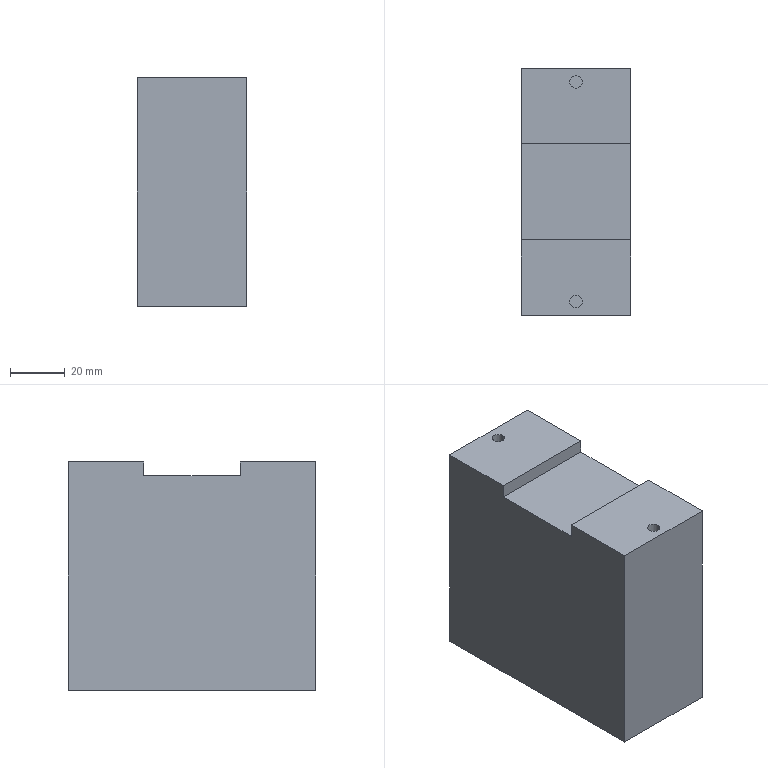Part | STEP file | BZJ-LSX-RGX PLC扩展IO FX5-16ET_ES8(输入,8输出,晶体管漏型) | 1 solid | 16 faces | box 40 x 90 x 83 mm | volume 291482 mm3 | plane 12 | cylinder 4 | commonest cylinder face diameters 4.5 x4
STEP:
#1=CARTESIAN_POINT('',(0.,0.,0.));
#2=DIRECTION('',(0.,0.,1.));
#3=DIRECTION('',(1.,0.,0.));
#4=AXIS2_PLACEMENT_3D('',#1,#2,#3);
#5=CARTESIAN_POINT('',(2.25,40.,31.5));
#6=VERTEX_POINT('',#5);
#7=CARTESIAN_POINT('',(2.25,40.,41.5));
#8=VERTEX_POINT('',#7);
#9=CARTESIAN_POINT('',(2.25,40.,31.5));
#10=DIRECTION('',(0.,0.,1.));
#11=VECTOR('',#10,1.);
#12=LINE('',#9,#11);
#13=CARTESIAN_POINT('',(0.,40.,31.5));
#14=DIRECTION('',(0.,0.,1.));
#15=DIRECTION('',(1.,0.,0.));
#16=AXIS2_PLACEMENT_3D('',#13,#14,#15);
#17=CYLINDRICAL_SURFACE('',#16,2.25);
#18=CARTESIAN_POINT('',(6.283,0.));
#19=DIRECTION('',(0.,1.));
#20=VECTOR('',#19,1.);
#21=LINE('',#18,#20);
#22=(GEOMETRIC_REPRESENTATION_CONTEXT(2)PARAMETRIC_REPRESENTATION_CONTEXT()REPRESENTATION_CONTEXT('',''));
#23=DEFINITIONAL_REPRESENTATION('',(#21),#22);
#24=PCURVE('',#17,#23);
#25=CARTESIAN_POINT('',(0.,40.,31.5));
#26=DIRECTION('',(0.,0.,1.));
#27=DIRECTION('',(1.,0.,0.));
#28=AXIS2_PLACEMENT_3D('',#25,#26,#27);
#29=CYLINDRICAL_SURFACE('',#28,2.25);
#30=CARTESIAN_POINT('',(0.,0.));
#31=DIRECTION('',(0.,1.));
#32=VECTOR('',#31,1.);
#33=LINE('',#30,#32);
#34=(GEOMETRIC_REPRESENTATION_CONTEXT(2)PARAMETRIC_REPRESENTATION_CONTEXT()REPRESENTATION_CONTEXT('',''));
#35=DEFINITIONAL_REPRESENTATION('',(#33),#34);
#36=PCURVE('',#29,#35);
#37=SURFACE_CURVE('',#12,(#24,#36),.PCURVE_S1.);
#38=EDGE_CURVE('',#6,#8,#37,.T.);
#39=ORIENTED_EDGE('',*,*,#38,.T.);
#40=CARTESIAN_POINT('',(-2.25,40.,41.5));
#41=VERTEX_POINT('',#40);
#42=CARTESIAN_POINT('',(0.,40.,41.5));
#43=DIRECTION('',(0.,0.,-1.));
#44=DIRECTION('',(-1.,0.,0.));
#45=AXIS2_PLACEMENT_3D('',#42,#43,#44);
#46=CIRCLE('',#45,2.25);
#47=CARTESIAN_POINT('',(9.425,10.));
#48=DIRECTION('',(-1.,0.));
#49=VECTOR('',#48,1.);
#50=LINE('',#47,#49);
#51=(GEOMETRIC_REPRESENTATION_CONTEXT(2)PARAMETRIC_REPRESENTATION_CONTEXT()REPRESENTATION_CONTEXT('',''));
#52=DEFINITIONAL_REPRESENTATION('',(#50),#51);
#53=PCURVE('',#17,#52);
#54=CARTESIAN_POINT('',(0.,0.,41.5));
#55=DIRECTION('',(0.,0.,-1.));
#56=DIRECTION('',(-1.,0.,0.));
#57=AXIS2_PLACEMENT_3D('',#54,#55,#56);
#58=PLANE('',#57);
#59=CARTESIAN_POINT('',(0.,40.));
#60=DIRECTION('',(1.,0.));
#61=AXIS2_PLACEMENT_2D('',#59,#60);
#62=CIRCLE('',#61,2.25);
#63=(GEOMETRIC_REPRESENTATION_CONTEXT(2)PARAMETRIC_REPRESENTATION_CONTEXT()REPRESENTATION_CONTEXT('',''));
#64=DEFINITIONAL_REPRESENTATION('',(#62),#63);
#65=PCURVE('',#58,#64);
#66=SURFACE_CURVE('',#46,(#53,#65),.PCURVE_S1.);
#67=EDGE_CURVE('',#8,#41,#66,.T.);
#68=ORIENTED_EDGE('',*,*,#67,.T.);
#69=CARTESIAN_POINT('',(-2.25,40.,31.5));
#70=VERTEX_POINT('',#69);
#71=CARTESIAN_POINT('',(-2.25,40.,31.5));
#72=DIRECTION('',(0.,0.,1.));
#73=VECTOR('',#72,1.);
#74=LINE('',#71,#73);
#75=CARTESIAN_POINT('',(3.142,0.));
#76=DIRECTION('',(0.,1.));
#77=VECTOR('',#76,1.);
#78=LINE('',#75,#77);
#79=(GEOMETRIC_REPRESENTATION_CONTEXT(2)PARAMETRIC_REPRESENTATION_CONTEXT()REPRESENTATION_CONTEXT('',''));
#80=DEFINITIONAL_REPRESENTATION('',(#78),#79);
#81=PCURVE('',#17,#80);
#82=CARTESIAN_POINT('',(3.142,0.));
#83=DIRECTION('',(0.,1.));
#84=VECTOR('',#83,1.);
#85=LINE('',#82,#84);
#86=(GEOMETRIC_REPRESENTATION_CONTEXT(2)PARAMETRIC_REPRESENTATION_CONTEXT()REPRESENTATION_CONTEXT('',''));
#87=DEFINITIONAL_REPRESENTATION('',(#85),#86);
#88=PCURVE('',#29,#87);
#89=SURFACE_CURVE('',#74,(#81,#88),.PCURVE_S1.);
#90=EDGE_CURVE('',#70,#41,#89,.T.);
#91=ORIENTED_EDGE('',*,*,#90,.F.);
#92=CARTESIAN_POINT('',(0.,40.,31.5));
#93=DIRECTION('',(0.,0.,-1.));
#94=DIRECTION('',(-1.,0.,0.));
#95=AXIS2_PLACEMENT_3D('',#92,#93,#94);
#96=CIRCLE('',#95,2.25);
#97=CARTESIAN_POINT('',(9.425,0.));
#98=DIRECTION('',(-1.,0.));
#99=VECTOR('',#98,1.);
#100=LINE('',#97,#99);
#101=(GEOMETRIC_REPRESENTATION_CONTEXT(2)PARAMETRIC_REPRESENTATION_CONTEXT()REPRESENTATION_CONTEXT('',''));
#102=DEFINITIONAL_REPRESENTATION('',(#100),#101);
#103=PCURVE('',#17,#102);
#104=CARTESIAN_POINT('',(0.,40.,31.5));
#105=DIRECTION('',(0.,0.,-1.));
#106=DIRECTION('',(-1.,0.,0.));
#107=AXIS2_PLACEMENT_3D('',#104,#105,#106);
#108=PLANE('',#107);
#109=CARTESIAN_POINT('',(0.,0.));
#110=DIRECTION('',(1.,0.));
#111=AXIS2_PLACEMENT_2D('',#109,#110);
#112=CIRCLE('',#111,2.25);
#113=(GEOMETRIC_REPRESENTATION_CONTEXT(2)PARAMETRIC_REPRESENTATION_CONTEXT()REPRESENTATION_CONTEXT('',''));
#114=DEFINITIONAL_REPRESENTATION('',(#112),#113);
#115=PCURVE('',#108,#114);
#116=SURFACE_CURVE('',#96,(#103,#115),.PCURVE_S1.);
#117=EDGE_CURVE('',#6,#70,#116,.T.);
#118=ORIENTED_EDGE('',*,*,#117,.F.);
#119=EDGE_LOOP('',(#39,#68,#91,#118));
#120=FACE_BOUND('',#119,.F.);
#121=ADVANCED_FACE('',(#120),#17,.F.);
#122=CARTESIAN_POINT('',(2.25,-40.,31.5));
#123=VERTEX_POINT('',#122);
#124=CARTESIAN_POINT('',(2.25,-40.,41.5));
#125=VERTEX_POINT('',#124);
#126=CARTESIAN_POINT('',(2.25,-40.,31.5));
#127=DIRECTION('',(0.,0.,1.));
#128=VECTOR('',#127,1.);
#129=LINE('',#126,#128);
#130=CARTESIAN_POINT('',(0.,-40.,31.5));
#131=DIRECTION('',(0.,0.,1.));
#132=DIRECTION('',(1.,0.,0.));
#133=AXIS2_PLACEMENT_3D('',#130,#131,#132);
#134=CYLINDRICAL_SURFACE('',#133,2.25);
#135=CARTESIAN_POINT('',(6.283,0.));
#136=DIRECTION('',(0.,1.));
#137=VECTOR('',#136,1.);
#138=LINE('',#135,#137);
#139=(GEOMETRIC_REPRESENTATION_CONTEXT(2)PARAMETRIC_REPRESENTATION_CONTEXT()REPRESENTATION_CONTEXT('',''));
#140=DEFINITIONAL_REPRESENTATION('',(#138),#139);
#141=PCURVE('',#134,#140);
#142=CARTESIAN_POINT('',(0.,-40.,31.5));
#143=DIRECTION('',(0.,0.,1.));
#144=DIRECTION('',(1.,0.,0.));
#145=AXIS2_PLACEMENT_3D('',#142,#143,#144);
#146=CYLINDRICAL_SURFACE('',#145,2.25);
#147=CARTESIAN_POINT('',(0.,0.));
#148=DIRECTION('',(0.,1.));
#149=VECTOR('',#148,1.);
#150=LINE('',#147,#149);
#151=(GEOMETRIC_REPRESENTATION_CONTEXT(2)PARAMETRIC_REPRESENTATION_CONTEXT()REPRESENTATION_CONTEXT('',''));
#152=DEFINITIONAL_REPRESENTATION('',(#150),#151);
#153=PCURVE('',#146,#152);
#154=SURFACE_CURVE('',#129,(#141,#153),.PCURVE_S1.);
#155=EDGE_CURVE('',#123,#125,#154,.T.);
#156=ORIENTED_EDGE('',*,*,#155,.T.);
#157=CARTESIAN_POINT('',(-2.25,-40.,41.5));
#158=VERTEX_POINT('',#157);
#159=CARTESIAN_POINT('',(0.,-40.,41.5));
#160=DIRECTION('',(0.,0.,-1.));
#161=DIRECTION('',(1.,0.,0.));
#162=AXIS2_PLACEMENT_3D('',#159,#160,#161);
#163=CIRCLE('',#162,2.25);
#164=CARTESIAN_POINT('',(6.283,10.));
#165=DIRECTION('',(-1.,0.));
#166=VECTOR('',#165,1.);
#167=LINE('',#164,#166);
#168=(GEOMETRIC_REPRESENTATION_CONTEXT(2)PARAMETRIC_REPRESENTATION_CONTEXT()REPRESENTATION_CONTEXT('',''));
#169=DEFINITIONAL_REPRESENTATION('',(#167),#168);
#170=PCURVE('',#134,#169);
#171=CARTESIAN_POINT('',(0.,0.,41.5));
#172=DIRECTION('',(0.,0.,-1.));
#173=DIRECTION('',(-1.,0.,0.));
#174=AXIS2_PLACEMENT_3D('',#171,#172,#173);
#175=PLANE('',#174);
#176=CARTESIAN_POINT('',(0.,-40.));
#177=DIRECTION('',(-1.,0.));
#178=AXIS2_PLACEMENT_2D('',#176,#177);
#179=CIRCLE('',#178,2.25);
#180=(GEOMETRIC_REPRESENTATION_CONTEXT(2)PARAMETRIC_REPRESENTATION_CONTEXT()REPRESENTATION_CONTEXT('',''));
#181=DEFINITIONAL_REPRESENTATION('',(#179),#180);
#182=PCURVE('',#175,#181);
#183=SURFACE_CURVE('',#163,(#170,#182),.PCURVE_S1.);
#184=EDGE_CURVE('',#125,#158,#183,.T.);
#185=ORIENTED_EDGE('',*,*,#184,.T.);
#186=CARTESIAN_POINT('',(-2.25,-40.,31.5));
#187=VERTEX_POINT('',#186);
#188=CARTESIAN_POINT('',(-2.25,-40.,31.5));
#189=DIRECTION('',(0.,0.,1.));
#190=VECTOR('',#189,1.);
#191=LINE('',#188,#190);
#192=CARTESIAN_POINT('',(3.142,0.));
#193=DIRECTION('',(0.,1.));
#194=VECTOR('',#193,1.);
#195=LINE('',#192,#194);
#196=(GEOMETRIC_REPRESENTATION_CONTEXT(2)PARAMETRIC_REPRESENTATION_CONTEXT()REPRESENTATION_CONTEXT('',''));
#197=DEFINITIONAL_REPRESENTATION('',(#195),#196);
#198=PCURVE('',#134,#197);
#199=CARTESIAN_POINT('',(3.142,0.));
#200=DIRECTION('',(0.,1.));
#201=VECTOR('',#200,1.);
#202=LINE('',#199,#201);
#203=(GEOMETRIC_REPRESENTATION_CONTEXT(2)PARAMETRIC_REPRESENTATION_CONTEXT()REPRESENTATION_CONTEXT('',''));
#204=DEFINITIONAL_REPRESENTATION('',(#202),#203);
#205=PCURVE('',#146,#204);
#206=SURFACE_CURVE('',#191,(#198,#205),.PCURVE_S1.);
#207=EDGE_CURVE('',#187,#158,#206,.T.);
#208=ORIENTED_EDGE('',*,*,#207,.F.);
#209=CARTESIAN_POINT('',(0.,-40.,31.5));
#210=DIRECTION('',(0.,0.,-1.));
#211=DIRECTION('',(1.,0.,0.));
#212=AXIS2_PLACEMENT_3D('',#209,#210,#211);
#213=CIRCLE('',#212,2.25);
#214=CARTESIAN_POINT('',(6.283,0.));
#215=DIRECTION('',(-1.,0.));
#216=VECTOR('',#215,1.);
#217=LINE('',#214,#216);
#218=(GEOMETRIC_REPRESENTATION_CONTEXT(2)PARAMETRIC_REPRESENTATION_CONTEXT()REPRESENTATION_CONTEXT('',''));
#219=DEFINITIONAL_REPRESENTATION('',(#217),#218);
#220=PCURVE('',#134,#219);
#221=CARTESIAN_POINT('',(0.,-40.,31.5));
#222=DIRECTION('',(0.,0.,1.));
#223=DIRECTION('',(1.,0.,0.));
#224=AXIS2_PLACEMENT_3D('',#221,#222,#223);
#225=PLANE('',#224);
#226=CARTESIAN_POINT('',(2.25,0.));
#227=CARTESIAN_POINT('',(2.25,-3.897));
#228=CARTESIAN_POINT('',(-1.125,-1.949));
#229=CARTESIAN_POINT('',(-4.5,0.));
#230=CARTESIAN_POINT('',(-1.125,1.949));
#231=CARTESIAN_POINT('',(2.25,3.897));
#232=CARTESIAN_POINT('',(2.25,0.));
#233=(BOUNDED_CURVE()B_SPLINE_CURVE(2,(#226,#227,#228,#229,#230,#231,#232),.UNSPECIFIED.,.T.,.F.)B_SPLINE_CURVE_WITH_KNOTS((1,2,2,2,2,1),(-2.094,0.,2.094,4.189,6.283,8.378),.UNSPECIFIED.)CURVE()GEOMETRIC_REPRESENTATION_ITEM()RATIONAL_B_SPLINE_CURVE((1.,0.5,1.,0.5,1.,0.5,1.))REPRESENTATION_ITEM(''));
#234=(GEOMETRIC_REPRESENTATION_CONTEXT(2)PARAMETRIC_REPRESENTATION_CONTEXT()REPRESENTATION_CONTEXT('',''));
#235=DEFINITIONAL_REPRESENTATION('',(#233),#234);
#236=PCURVE('',#225,#235);
#237=SURFACE_CURVE('',#213,(#220,#236),.PCURVE_S1.);
#238=EDGE_CURVE('',#123,#187,#237,.T.);
#239=ORIENTED_EDGE('',*,*,#238,.F.);
#240=EDGE_LOOP('',(#156,#185,#208,#239));
#241=FACE_BOUND('',#240,.F.);
#242=ADVANCED_FACE('',(#241),#134,.F.);
#243=ORIENTED_EDGE('',*,*,#67,.T.);
#244=CARTESIAN_POINT('',(0.,40.,41.5));
#245=DIRECTION('',(0.,0.,-1.));
#246=DIRECTION('',(-1.,0.,0.));
#247=AXIS2_PLACEMENT_3D('',#244,#245,#246);
#248=CIRCLE('',#247,2.25);
#249=CARTESIAN_POINT('',(0.,40.));
#250=DIRECTION('',(1.,0.));
#251=AXIS2_PLACEMENT_2D('',#249,#250);
#252=CIRCLE('',#251,2.25);
#253=(GEOMETRIC_REPRESENTATION_CONTEXT(2)PARAMETRIC_REPRESENTATION_CONTEXT()REPRESENTATION_CONTEXT('',''));
#254=DEFINITIONAL_REPRESENTATION('',(#252),#253);
#255=PCURVE('',#58,#254);
#256=CARTESIAN_POINT('',(3.142,10.));
#257=DIRECTION('',(-1.,0.));
#258=VECTOR('',#257,1.);
#259=LINE('',#256,#258);
#260=(GEOMETRIC_REPRESENTATION_CONTEXT(2)PARAMETRIC_REPRESENTATION_CONTEXT()REPRESENTATION_CONTEXT('',''));
#261=DEFINITIONAL_REPRESENTATION('',(#259),#260);
#262=PCURVE('',#29,#261);
#263=SURFACE_CURVE('',#248,(#255,#262),.PCURVE_S1.);
#264=EDGE_CURVE('',#41,#8,#263,.T.);
#265=ORIENTED_EDGE('',*,*,#264,.T.);
#266=EDGE_LOOP('',(#243,#265));
#267=FACE_BOUND('',#266,.T.);
#268=CARTESIAN_POINT('',(-20.,45.,41.5));
#269=VERTEX_POINT('',#268);
#270=CARTESIAN_POINT('',(-20.,17.5,41.5));
#271=VERTEX_POINT('',#270);
#272=CARTESIAN_POINT('',(-20.,45.,41.5));
#273=DIRECTION('',(0.,-1.,0.));
#274=VECTOR('',#273,1.);
#275=LINE('',#272,#274);
#276=CARTESIAN_POINT('',(20.,45.));
#277=DIRECTION('',(0.,-1.));
#278=VECTOR('',#277,1.);
#279=LINE('',#276,#278);
#280=(GEOMETRIC_REPRESENTATION_CONTEXT(2)PARAMETRIC_REPRESENTATION_CONTEXT()REPRESENTATION_CONTEXT('',''));
#281=DEFINITIONAL_REPRESENTATION('',(#279),#280);
#282=PCURVE('',#58,#281);
#283=CARTESIAN_POINT('',(-20.,45.,41.5));
#284=DIRECTION('',(1.,0.,0.));
#285=DIRECTION('',(0.,1.,0.));
#286=AXIS2_PLACEMENT_3D('',#283,#284,#285);
#287=PLANE('',#286);
#288=CARTESIAN_POINT('',(0.,0.));
#289=DIRECTION('',(-1.,0.));
#290=VECTOR('',#289,1.);
#291=LINE('',#288,#290);
#292=(GEOMETRIC_REPRESENTATION_CONTEXT(2)PARAMETRIC_REPRESENTATION_CONTEXT()REPRESENTATION_CONTEXT('',''));
#293=DEFINITIONAL_REPRESENTATION('',(#291),#292);
#294=PCURVE('',#287,#293);
#295=SURFACE_CURVE('',#275,(#282,#294),.PCURVE_S1.);
#296=EDGE_CURVE('',#269,#271,#295,.T.);
#297=ORIENTED_EDGE('',*,*,#296,.T.);
#298=CARTESIAN_POINT('',(20.,17.5,41.5));
#299=VERTEX_POINT('',#298);
#300=CARTESIAN_POINT('',(0.,17.5,41.5));
#301=DIRECTION('',(1.,0.,0.));
#302=VECTOR('',#301,1.);
#303=LINE('',#300,#302);
#304=CARTESIAN_POINT('',(0.,17.5));
#305=DIRECTION('',(-1.,0.));
#306=VECTOR('',#305,1.);
#307=LINE('',#304,#306);
#308=(GEOMETRIC_REPRESENTATION_CONTEXT(2)PARAMETRIC_REPRESENTATION_CONTEXT()REPRESENTATION_CONTEXT('',''));
#309=DEFINITIONAL_REPRESENTATION('',(#307),#308);
#310=PCURVE('',#58,#309);
#311=CARTESIAN_POINT('',(-20.,17.5,36.5));
#312=DIRECTION('',(0.,1.,0.));
#313=DIRECTION('',(-1.,0.,0.));
#314=AXIS2_PLACEMENT_3D('',#311,#312,#313);
#315=PLANE('',#314);
#316=CARTESIAN_POINT('',(-20.,5.));
#317=DIRECTION('',(-1.,0.));
#318=VECTOR('',#317,1.);
#319=LINE('',#316,#318);
#320=(GEOMETRIC_REPRESENTATION_CONTEXT(2)PARAMETRIC_REPRESENTATION_CONTEXT()REPRESENTATION_CONTEXT('',''));
#321=DEFINITIONAL_REPRESENTATION('',(#319),#320);
#322=PCURVE('',#315,#321);
#323=SURFACE_CURVE('',#303,(#310,#322),.PCURVE_S1.);
#324=EDGE_CURVE('',#271,#299,#323,.T.);
#325=ORIENTED_EDGE('',*,*,#324,.T.);
#326=CARTESIAN_POINT('',(20.,45.,41.5));
#327=VERTEX_POINT('',#326);
#328=CARTESIAN_POINT('',(20.,45.,41.5));
#329=DIRECTION('',(0.,1.,0.));
#330=VECTOR('',#329,1.);
#331=LINE('',#328,#330);
#332=CARTESIAN_POINT('',(-20.,45.));
#333=DIRECTION('',(0.,1.));
#334=VECTOR('',#333,1.);
#335=LINE('',#332,#334);
#336=(GEOMETRIC_REPRESENTATION_CONTEXT(2)PARAMETRIC_REPRESENTATION_CONTEXT()REPRESENTATION_CONTEXT('',''));
#337=DEFINITIONAL_REPRESENTATION('',(#335),#336);
#338=PCURVE('',#58,#337);
#339=CARTESIAN_POINT('',(20.,45.,41.5));
#340=DIRECTION('',(-1.,0.,0.));
#341=DIRECTION('',(0.,-1.,0.));
#342=AXIS2_PLACEMENT_3D('',#339,#340,#341);
#343=PLANE('',#342);
#344=CARTESIAN_POINT('',(0.,0.));
#345=DIRECTION('',(-1.,0.));
#346=VECTOR('',#345,1.);
#347=LINE('',#344,#346);
#348=(GEOMETRIC_REPRESENTATION_CONTEXT(2)PARAMETRIC_REPRESENTATION_CONTEXT()REPRESENTATION_CONTEXT('',''));
#349=DEFINITIONAL_REPRESENTATION('',(#347),#348);
#350=PCURVE('',#343,#349);
#351=SURFACE_CURVE('',#331,(#338,#350),.PCURVE_S1.);
#352=EDGE_CURVE('',#299,#327,#351,.T.);
#353=ORIENTED_EDGE('',*,*,#352,.T.);
#354=CARTESIAN_POINT('',(20.,45.,41.5));
#355=DIRECTION('',(-1.,0.,0.));
#356=VECTOR('',#355,1.);
#357=LINE('',#354,#356);
#358=CARTESIAN_POINT('',(-20.,45.));
#359=DIRECTION('',(1.,0.));
#360=VECTOR('',#359,1.);
#361=LINE('',#358,#360);
#362=(GEOMETRIC_REPRESENTATION_CONTEXT(2)PARAMETRIC_REPRESENTATION_CONTEXT()REPRESENTATION_CONTEXT('',''));
#363=DEFINITIONAL_REPRESENTATION('',(#361),#362);
#364=PCURVE('',#58,#363);
#365=CARTESIAN_POINT('',(20.,45.,41.5));
#366=DIRECTION('',(0.,-1.,0.));
#367=DIRECTION('',(0.,0.,-1.));
#368=AXIS2_PLACEMENT_3D('',#365,#366,#367);
#369=PLANE('',#368);
#370=CARTESIAN_POINT('',(0.,0.));
#371=DIRECTION('',(0.,-1.));
#372=VECTOR('',#371,1.);
#373=LINE('',#370,#372);
#374=(GEOMETRIC_REPRESENTATION_CONTEXT(2)PARAMETRIC_REPRESENTATION_CONTEXT()REPRESENTATION_CONTEXT('',''));
#375=DEFINITIONAL_REPRESENTATION('',(#373),#374);
#376=PCURVE('',#369,#375);
#377=SURFACE_CURVE('',#357,(#364,#376),.PCURVE_S1.);
#378=EDGE_CURVE('',#327,#269,#377,.T.);
#379=ORIENTED_EDGE('',*,*,#378,.T.);
#380=EDGE_LOOP('',(#297,#325,#353,#379));
#381=FACE_BOUND('',#380,.T.);
#382=ADVANCED_FACE('',(#267,#381),#58,.F.);
#383=CARTESIAN_POINT('',(-20.,-17.5,36.5));
#384=VERTEX_POINT('',#383);
#385=CARTESIAN_POINT('',(-20.,17.5,36.5));
#386=VERTEX_POINT('',#385);
#387=CARTESIAN_POINT('',(-20.,17.5,36.5));
#388=DIRECTION('',(0.,1.,0.));
#389=VECTOR('',#388,1.);
#390=LINE('',#387,#389);
#391=CARTESIAN_POINT('',(-27.5,-5.));
#392=DIRECTION('',(1.,0.));
#393=VECTOR('',#392,1.);
#394=LINE('',#391,#393);
#395=(GEOMETRIC_REPRESENTATION_CONTEXT(2)PARAMETRIC_REPRESENTATION_CONTEXT()REPRESENTATION_CONTEXT('',''));
#396=DEFINITIONAL_REPRESENTATION('',(#394),#395);
#397=PCURVE('',#287,#396);
#398=CARTESIAN_POINT('',(-20.,17.5,36.5));
#399=DIRECTION('',(0.,0.,-1.));
#400=DIRECTION('',(-1.,0.,0.));
#401=AXIS2_PLACEMENT_3D('',#398,#399,#400);
#402=PLANE('',#401);
#403=CARTESIAN_POINT('',(0.,0.));
#404=DIRECTION('',(0.,1.));
#405=VECTOR('',#404,1.);
#406=LINE('',#403,#405);
#407=(GEOMETRIC_REPRESENTATION_CONTEXT(2)PARAMETRIC_REPRESENTATION_CONTEXT()REPRESENTATION_CONTEXT('',''));
#408=DEFINITIONAL_REPRESENTATION('',(#406),#407);
#409=PCURVE('',#402,#408);
#410=SURFACE_CURVE('',#390,(#397,#409),.PCURVE_S1.);
#411=EDGE_CURVE('',#384,#386,#410,.T.);
#412=ORIENTED_EDGE('',*,*,#411,.T.);
#413=CARTESIAN_POINT('',(-20.,17.5,36.5));
#414=DIRECTION('',(0.,0.,1.));
#415=VECTOR('',#414,1.);
#416=LINE('',#413,#415);
#417=CARTESIAN_POINT('',(-27.5,-5.));
#418=DIRECTION('',(0.,1.));
#419=VECTOR('',#418,1.);
#420=LINE('',#417,#419);
#421=(GEOMETRIC_REPRESENTATION_CONTEXT(2)PARAMETRIC_REPRESENTATION_CONTEXT()REPRESENTATION_CONTEXT('',''));
#422=DEFINITIONAL_REPRESENTATION('',(#420),#421);
#423=PCURVE('',#287,#422);
#424=CARTESIAN_POINT('',(0.,0.));
#425=DIRECTION('',(0.,1.));
#426=VECTOR('',#425,1.);
#427=LINE('',#424,#426);
#428=(GEOMETRIC_REPRESENTATION_CONTEXT(2)PARAMETRIC_REPRESENTATION_CONTEXT()REPRESENTATION_CONTEXT('',''));
#429=DEFINITIONAL_REPRESENTATION('',(#427),#428);
#430=PCURVE('',#315,#429);
#431=SURFACE_CURVE('',#416,(#423,#430),.PCURVE_S1.);
#432=EDGE_CURVE('',#386,#271,#431,.T.);
#433=ORIENTED_EDGE('',*,*,#432,.T.);
#434=ORIENTED_EDGE('',*,*,#296,.F.);
#435=CARTESIAN_POINT('',(-20.,45.,-41.5));
#436=VERTEX_POINT('',#435);
#437=CARTESIAN_POINT('',(-20.,45.,41.5));
#438=DIRECTION('',(0.,0.,-1.));
#439=VECTOR('',#438,1.);
#440=LINE('',#437,#439);
#441=CARTESIAN_POINT('',(0.,0.));
#442=DIRECTION('',(0.,-1.));
#443=VECTOR('',#442,1.);
#444=LINE('',#441,#443);
#445=(GEOMETRIC_REPRESENTATION_CONTEXT(2)PARAMETRIC_REPRESENTATION_CONTEXT()REPRESENTATION_CONTEXT('',''));
#446=DEFINITIONAL_REPRESENTATION('',(#444),#445);
#447=PCURVE('',#287,#446);
#448=CARTESIAN_POINT('',(0.,-40.));
#449=DIRECTION('',(1.,0.));
#450=VECTOR('',#449,1.);
#451=LINE('',#448,#450);
#452=(GEOMETRIC_REPRESENTATION_CONTEXT(2)PARAMETRIC_REPRESENTATION_CONTEXT()REPRESENTATION_CONTEXT('',''));
#453=DEFINITIONAL_REPRESENTATION('',(#451),#452);
#454=PCURVE('',#369,#453);
#455=SURFACE_CURVE('',#440,(#447,#454),.PCURVE_S1.);
#456=EDGE_CURVE('',#269,#436,#455,.T.);
#457=ORIENTED_EDGE('',*,*,#456,.T.);
#458=CARTESIAN_POINT('',(-20.,-45.,-41.5));
#459=VERTEX_POINT('',#458);
#460=CARTESIAN_POINT('',(-20.,45.,-41.5));
#461=DIRECTION('',(0.,-1.,0.));
#462=VECTOR('',#461,1.);
#463=LINE('',#460,#462);
#464=CARTESIAN_POINT('',(0.,-83.));
#465=DIRECTION('',(-1.,0.));
#466=VECTOR('',#465,1.);
#467=LINE('',#464,#466);
#468=(GEOMETRIC_REPRESENTATION_CONTEXT(2)PARAMETRIC_REPRESENTATION_CONTEXT()REPRESENTATION_CONTEXT('',''));
#469=DEFINITIONAL_REPRESENTATION('',(#467),#468);
#470=PCURVE('',#287,#469);
#471=CARTESIAN_POINT('',(0.,0.,-41.5));
#472=DIRECTION('',(0.,0.,-1.));
#473=DIRECTION('',(-1.,0.,0.));
#474=AXIS2_PLACEMENT_3D('',#471,#472,#473);
#475=PLANE('',#474);
#476=CARTESIAN_POINT('',(20.,45.));
#477=DIRECTION('',(0.,-1.));
#478=VECTOR('',#477,1.);
#479=LINE('',#476,#478);
#480=(GEOMETRIC_REPRESENTATION_CONTEXT(2)PARAMETRIC_REPRESENTATION_CONTEXT()REPRESENTATION_CONTEXT('',''));
#481=DEFINITIONAL_REPRESENTATION('',(#479),#480);
#482=PCURVE('',#475,#481);
#483=SURFACE_CURVE('',#463,(#470,#482),.PCURVE_S1.);
#484=EDGE_CURVE('',#436,#459,#483,.T.);
#485=ORIENTED_EDGE('',*,*,#484,.T.);
#486=CARTESIAN_POINT('',(-20.,-45.,41.5));
#487=VERTEX_POINT('',#486);
#488=CARTESIAN_POINT('',(-20.,-45.,41.5));
#489=DIRECTION('',(0.,0.,-1.));
#490=VECTOR('',#489,1.);
#491=LINE('',#488,#490);
#492=CARTESIAN_POINT('',(-90.,0.));
#493=DIRECTION('',(0.,-1.));
#494=VECTOR('',#493,1.);
#495=LINE('',#492,#494);
#496=(GEOMETRIC_REPRESENTATION_CONTEXT(2)PARAMETRIC_REPRESENTATION_CONTEXT()REPRESENTATION_CONTEXT('',''));
#497=DEFINITIONAL_REPRESENTATION('',(#495),#496);
#498=PCURVE('',#287,#497);
#499=CARTESIAN_POINT('',(20.,-45.,41.5));
#500=DIRECTION('',(0.,1.,0.));
#501=DIRECTION('',(-1.,0.,0.));
#502=AXIS2_PLACEMENT_3D('',#499,#500,#501);
#503=PLANE('',#502);
#504=CARTESIAN_POINT('',(40.,0.));
#505=DIRECTION('',(0.,-1.));
#506=VECTOR('',#505,1.);
#507=LINE('',#504,#506);
#508=(GEOMETRIC_REPRESENTATION_CONTEXT(2)PARAMETRIC_REPRESENTATION_CONTEXT()REPRESENTATION_CONTEXT('',''));
#509=DEFINITIONAL_REPRESENTATION('',(#507),#508);
#510=PCURVE('',#503,#509);
#511=SURFACE_CURVE('',#491,(#498,#510),.PCURVE_S1.);
#512=EDGE_CURVE('',#487,#459,#511,.T.);
#513=ORIENTED_EDGE('',*,*,#512,.F.);
#514=CARTESIAN_POINT('',(-20.,-17.5,41.5));
#515=VERTEX_POINT('',#514);
#516=CARTESIAN_POINT('',(-20.,45.,41.5));
#517=DIRECTION('',(0.,-1.,0.));
#518=VECTOR('',#517,1.);
#519=LINE('',#516,#518);
#520=CARTESIAN_POINT('',(0.,0.));
#521=DIRECTION('',(-1.,0.));
#522=VECTOR('',#521,1.);
#523=LINE('',#520,#522);
#524=(GEOMETRIC_REPRESENTATION_CONTEXT(2)PARAMETRIC_REPRESENTATION_CONTEXT()REPRESENTATION_CONTEXT('',''));
#525=DEFINITIONAL_REPRESENTATION('',(#523),#524);
#526=PCURVE('',#287,#525);
#527=CARTESIAN_POINT('',(20.,45.));
#528=DIRECTION('',(0.,-1.));
#529=VECTOR('',#528,1.);
#530=LINE('',#527,#529);
#531=(GEOMETRIC_REPRESENTATION_CONTEXT(2)PARAMETRIC_REPRESENTATION_CONTEXT()REPRESENTATION_CONTEXT('',''));
#532=DEFINITIONAL_REPRESENTATION('',(#530),#531);
#533=PCURVE('',#175,#532);
#534=SURFACE_CURVE('',#519,(#526,#533),.PCURVE_S1.);
#535=EDGE_CURVE('',#515,#487,#534,.T.);
#536=ORIENTED_EDGE('',*,*,#535,.F.);
#537=CARTESIAN_POINT('',(-20.,-17.5,36.5));
#538=DIRECTION('',(0.,0.,-1.));
#539=VECTOR('',#538,1.);
#540=LINE('',#537,#539);
#541=CARTESIAN_POINT('',(-62.5,-5.));
#542=DIRECTION('',(0.,-1.));
#543=VECTOR('',#542,1.);
#544=LINE('',#541,#543);
#545=(GEOMETRIC_REPRESENTATION_CONTEXT(2)PARAMETRIC_REPRESENTATION_CONTEXT()REPRESENTATION_CONTEXT('',''));
#546=DEFINITIONAL_REPRESENTATION('',(#544),#545);
#547=PCURVE('',#287,#546);
#548=CARTESIAN_POINT('',(-20.,-17.5,36.5));
#549=DIRECTION('',(0.,-1.,0.));
#550=DIRECTION('',(1.,0.,0.));
#551=AXIS2_PLACEMENT_3D('',#548,#549,#550);
#552=PLANE('',#551);
#553=CARTESIAN_POINT('',(0.,0.));
#554=DIRECTION('',(0.,-1.));
#555=VECTOR('',#554,1.);
#556=LINE('',#553,#555);
#557=(GEOMETRIC_REPRESENTATION_CONTEXT(2)PARAMETRIC_REPRESENTATION_CONTEXT()REPRESENTATION_CONTEXT('',''));
#558=DEFINITIONAL_REPRESENTATION('',(#556),#557);
#559=PCURVE('',#552,#558);
#560=SURFACE_CURVE('',#540,(#547,#559),.PCURVE_S1.);
#561=EDGE_CURVE('',#515,#384,#560,.T.);
#562=ORIENTED_EDGE('',*,*,#561,.T.);
#563=EDGE_LOOP('',(#412,#433,#434,#457,#485,#513,#536,#562));
#564=FACE_BOUND('',#563,.T.);
#565=ADVANCED_FACE('',(#564),#287,.F.);
#566=CARTESIAN_POINT('',(20.,-45.,-41.5));
#567=VERTEX_POINT('',#566);
#568=CARTESIAN_POINT('',(20.,-45.,-41.5));
#569=DIRECTION('',(1.,0.,0.));
#570=VECTOR('',#569,1.);
#571=LINE('',#568,#570);
#572=CARTESIAN_POINT('',(0.,-83.));
#573=DIRECTION('',(-1.,0.));
#574=VECTOR('',#573,1.);
#575=LINE('',#572,#574);
#576=(GEOMETRIC_REPRESENTATION_CONTEXT(2)PARAMETRIC_REPRESENTATION_CONTEXT()REPRESENTATION_CONTEXT('',''));
#577=DEFINITIONAL_REPRESENTATION('',(#575),#576);
#578=PCURVE('',#503,#577);
#579=CARTESIAN_POINT('',(-20.,-45.));
#580=DIRECTION('',(-1.,0.));
#581=VECTOR('',#580,1.);
#582=LINE('',#579,#581);
#583=(GEOMETRIC_REPRESENTATION_CONTEXT(2)PARAMETRIC_REPRESENTATION_CONTEXT()REPRESENTATION_CONTEXT('',''));
#584=DEFINITIONAL_REPRESENTATION('',(#582),#583);
#585=PCURVE('',#475,#584);
#586=SURFACE_CURVE('',#571,(#578,#585),.PCURVE_S1.);
#587=EDGE_CURVE('',#459,#567,#586,.T.);
#588=ORIENTED_EDGE('',*,*,#587,.T.);
#589=CARTESIAN_POINT('',(20.,-45.,41.5));
#590=VERTEX_POINT('',#589);
#591=CARTESIAN_POINT('',(20.,-45.,41.5));
#592=DIRECTION('',(0.,0.,-1.));
#593=VECTOR('',#592,1.);
#594=LINE('',#591,#593);
#595=CARTESIAN_POINT('',(0.,0.));
#596=DIRECTION('',(0.,-1.));
#597=VECTOR('',#596,1.);
#598=LINE('',#595,#597);
#599=(GEOMETRIC_REPRESENTATION_CONTEXT(2)PARAMETRIC_REPRESENTATION_CONTEXT()REPRESENTATION_CONTEXT('',''));
#600=DEFINITIONAL_REPRESENTATION('',(#598),#599);
#601=PCURVE('',#503,#600);
#602=CARTESIAN_POINT('',(90.,0.));
#603=DIRECTION('',(0.,-1.));
#604=VECTOR('',#603,1.);
#605=LINE('',#602,#604);
#606=(GEOMETRIC_REPRESENTATION_CONTEXT(2)PARAMETRIC_REPRESENTATION_CONTEXT()REPRESENTATION_CONTEXT('',''));
#607=DEFINITIONAL_REPRESENTATION('',(#605),#606);
#608=PCURVE('',#343,#607);
#609=SURFACE_CURVE('',#594,(#601,#608),.PCURVE_S1.);
#610=EDGE_CURVE('',#590,#567,#609,.T.);
#611=ORIENTED_EDGE('',*,*,#610,.F.);
#612=CARTESIAN_POINT('',(20.,-45.,41.5));
#613=DIRECTION('',(1.,0.,0.));
#614=VECTOR('',#613,1.);
#615=LINE('',#612,#614);
#616=CARTESIAN_POINT('',(0.,0.));
#617=DIRECTION('',(-1.,0.));
#618=VECTOR('',#617,1.);
#619=LINE('',#616,#618);
#620=(GEOMETRIC_REPRESENTATION_CONTEXT(2)PARAMETRIC_REPRESENTATION_CONTEXT()REPRESENTATION_CONTEXT('',''));
#621=DEFINITIONAL_REPRESENTATION('',(#619),#620);
#622=PCURVE('',#503,#621);
#623=CARTESIAN_POINT('',(-20.,-45.));
#624=DIRECTION('',(-1.,0.));
#625=VECTOR('',#624,1.);
#626=LINE('',#623,#625);
#627=(GEOMETRIC_REPRESENTATION_CONTEXT(2)PARAMETRIC_REPRESENTATION_CONTEXT()REPRESENTATION_CONTEXT('',''));
#628=DEFINITIONAL_REPRESENTATION('',(#626),#627);
#629=PCURVE('',#175,#628);
#630=SURFACE_CURVE('',#615,(#622,#629),.PCURVE_S1.);
#631=EDGE_CURVE('',#487,#590,#630,.T.);
#632=ORIENTED_EDGE('',*,*,#631,.F.);
#633=ORIENTED_EDGE('',*,*,#512,.T.);
#634=EDGE_LOOP('',(#588,#611,#632,#633));
#635=FACE_BOUND('',#634,.T.);
#636=ADVANCED_FACE('',(#635),#503,.F.);
#637=ORIENTED_EDGE('',*,*,#352,.F.);
#638=CARTESIAN_POINT('',(20.,17.5,36.5));
#639=VERTEX_POINT('',#638);
#640=CARTESIAN_POINT('',(20.,17.5,36.5));
#641=DIRECTION('',(0.,0.,1.));
#642=VECTOR('',#641,1.);
#643=LINE('',#640,#642);
#644=CARTESIAN_POINT('',(27.5,-5.));
#645=DIRECTION('',(0.,1.));
#646=VECTOR('',#645,1.);
#647=LINE('',#644,#646);
#648=(GEOMETRIC_REPRESENTATION_CONTEXT(2)PARAMETRIC_REPRESENTATION_CONTEXT()REPRESENTATION_CONTEXT('',''));
#649=DEFINITIONAL_REPRESENTATION('',(#647),#648);
#650=PCURVE('',#343,#649);
#651=CARTESIAN_POINT('',(-40.,0.));
#652=DIRECTION('',(0.,1.));
#653=VECTOR('',#652,1.);
#654=LINE('',#651,#653);
#655=(GEOMETRIC_REPRESENTATION_CONTEXT(2)PARAMETRIC_REPRESENTATION_CONTEXT()REPRESENTATION_CONTEXT('',''));
#656=DEFINITIONAL_REPRESENTATION('',(#654),#655);
#657=PCURVE('',#315,#656);
#658=SURFACE_CURVE('',#643,(#650,#657),.PCURVE_S1.);
#659=EDGE_CURVE('',#639,#299,#658,.T.);
#660=ORIENTED_EDGE('',*,*,#659,.F.);
#661=CARTESIAN_POINT('',(20.,-17.5,36.5));
#662=VERTEX_POINT('',#661);
#663=CARTESIAN_POINT('',(20.,17.5,36.5));
#664=DIRECTION('',(0.,1.,0.));
#665=VECTOR('',#664,1.);
#666=LINE('',#663,#665);
#667=CARTESIAN_POINT('',(27.5,-5.));
#668=DIRECTION('',(-1.,0.));
#669=VECTOR('',#668,1.);
#670=LINE('',#667,#669);
#671=(GEOMETRIC_REPRESENTATION_CONTEXT(2)PARAMETRIC_REPRESENTATION_CONTEXT()REPRESENTATION_CONTEXT('',''));
#672=DEFINITIONAL_REPRESENTATION('',(#670),#671);
#673=PCURVE('',#343,#672);
#674=CARTESIAN_POINT('',(-40.,0.));
#675=DIRECTION('',(0.,1.));
#676=VECTOR('',#675,1.);
#677=LINE('',#674,#676);
#678=(GEOMETRIC_REPRESENTATION_CONTEXT(2)PARAMETRIC_REPRESENTATION_CONTEXT()REPRESENTATION_CONTEXT('',''));
#679=DEFINITIONAL_REPRESENTATION('',(#677),#678);
#680=PCURVE('',#402,#679);
#681=SURFACE_CURVE('',#666,(#673,#680),.PCURVE_S1.);
#682=EDGE_CURVE('',#662,#639,#681,.T.);
#683=ORIENTED_EDGE('',*,*,#682,.F.);
#684=CARTESIAN_POINT('',(20.,-17.5,41.5));
#685=VERTEX_POINT('',#684);
#686=CARTESIAN_POINT('',(20.,-17.5,36.5));
#687=DIRECTION('',(0.,0.,-1.));
#688=VECTOR('',#687,1.);
#689=LINE('',#686,#688);
#690=CARTESIAN_POINT('',(62.5,-5.));
#691=DIRECTION('',(0.,-1.));
#692=VECTOR('',#691,1.);
#693=LINE('',#690,#692);
#694=(GEOMETRIC_REPRESENTATION_CONTEXT(2)PARAMETRIC_REPRESENTATION_CONTEXT()REPRESENTATION_CONTEXT('',''));
#695=DEFINITIONAL_REPRESENTATION('',(#693),#694);
#696=PCURVE('',#343,#695);
#697=CARTESIAN_POINT('',(40.,0.));
#698=DIRECTION('',(0.,-1.));
#699=VECTOR('',#698,1.);
#700=LINE('',#697,#699);
#701=(GEOMETRIC_REPRESENTATION_CONTEXT(2)PARAMETRIC_REPRESENTATION_CONTEXT()REPRESENTATION_CONTEXT('',''));
#702=DEFINITIONAL_REPRESENTATION('',(#700),#701);
#703=PCURVE('',#552,#702);
#704=SURFACE_CURVE('',#689,(#696,#703),.PCURVE_S1.);
#705=EDGE_CURVE('',#685,#662,#704,.T.);
#706=ORIENTED_EDGE('',*,*,#705,.F.);
#707=CARTESIAN_POINT('',(20.,45.,41.5));
#708=DIRECTION('',(0.,1.,0.));
#709=VECTOR('',#708,1.);
#710=LINE('',#707,#709);
#711=CARTESIAN_POINT('',(0.,0.));
#712=DIRECTION('',(-1.,0.));
#713=VECTOR('',#712,1.);
#714=LINE('',#711,#713);
#715=(GEOMETRIC_REPRESENTATION_CONTEXT(2)PARAMETRIC_REPRESENTATION_CONTEXT()REPRESENTATION_CONTEXT('',''));
#716=DEFINITIONAL_REPRESENTATION('',(#714),#715);
#717=PCURVE('',#343,#716);
#718=CARTESIAN_POINT('',(-20.,45.));
#719=DIRECTION('',(0.,1.));
#720=VECTOR('',#719,1.);
#721=LINE('',#718,#720);
#722=(GEOMETRIC_REPRESENTATION_CONTEXT(2)PARAMETRIC_REPRESENTATION_CONTEXT()REPRESENTATION_CONTEXT('',''));
#723=DEFINITIONAL_REPRESENTATION('',(#721),#722);
#724=PCURVE('',#175,#723);
#725=SURFACE_CURVE('',#710,(#717,#724),.PCURVE_S1.);
#726=EDGE_CURVE('',#590,#685,#725,.T.);
#727=ORIENTED_EDGE('',*,*,#726,.F.);
#728=ORIENTED_EDGE('',*,*,#610,.T.);
#729=CARTESIAN_POINT('',(20.,45.,-41.5));
#730=VERTEX_POINT('',#729);
#731=CARTESIAN_POINT('',(20.,45.,-41.5));
#732=DIRECTION('',(0.,1.,0.));
#733=VECTOR('',#732,1.);
#734=LINE('',#731,#733);
#735=CARTESIAN_POINT('',(0.,-83.));
#736=DIRECTION('',(-1.,0.));
#737=VECTOR('',#736,1.);
#738=LINE('',#735,#737);
#739=(GEOMETRIC_REPRESENTATION_CONTEXT(2)PARAMETRIC_REPRESENTATION_CONTEXT()REPRESENTATION_CONTEXT('',''));
#740=DEFINITIONAL_REPRESENTATION('',(#738),#739);
#741=PCURVE('',#343,#740);
#742=CARTESIAN_POINT('',(-20.,45.));
#743=DIRECTION('',(0.,1.));
#744=VECTOR('',#743,1.);
#745=LINE('',#742,#744);
#746=(GEOMETRIC_REPRESENTATION_CONTEXT(2)PARAMETRIC_REPRESENTATION_CONTEXT()REPRESENTATION_CONTEXT('',''));
#747=DEFINITIONAL_REPRESENTATION('',(#745),#746);
#748=PCURVE('',#475,#747);
#749=SURFACE_CURVE('',#734,(#741,#748),.PCURVE_S1.);
#750=EDGE_CURVE('',#567,#730,#749,.T.);
#751=ORIENTED_EDGE('',*,*,#750,.T.);
#752=CARTESIAN_POINT('',(20.,45.,41.5));
#753=DIRECTION('',(0.,0.,-1.));
#754=VECTOR('',#753,1.);
#755=LINE('',#752,#754);
#756=CARTESIAN_POINT('',(0.,0.));
#757=DIRECTION('',(0.,-1.));
#758=VECTOR('',#757,1.);
#759=LINE('',#756,#758);
#760=(GEOMETRIC_REPRESENTATION_CONTEXT(2)PARAMETRIC_REPRESENTATION_CONTEXT()REPRESENTATION_CONTEXT('',''));
#761=DEFINITIONAL_REPRESENTATION('',(#759),#760);
#762=PCURVE('',#343,#761);
#763=CARTESIAN_POINT('',(0.,0.));
#764=DIRECTION('',(1.,0.));
#765=VECTOR('',#764,1.);
#766=LINE('',#763,#765);
#767=(GEOMETRIC_REPRESENTATION_CONTEXT(2)PARAMETRIC_REPRESENTATION_CONTEXT()REPRESENTATION_CONTEXT('',''));
#768=DEFINITIONAL_REPRESENTATION('',(#766),#767);
#769=PCURVE('',#369,#768);
#770=SURFACE_CURVE('',#755,(#762,#769),.PCURVE_S1.);
#771=EDGE_CURVE('',#327,#730,#770,.T.);
#772=ORIENTED_EDGE('',*,*,#771,.F.);
#773=EDGE_LOOP('',(#637,#660,#683,#706,#727,#728,#751,#772));
#774=FACE_BOUND('',#773,.T.);
#775=ADVANCED_FACE('',(#774),#343,.F.);
#776=CARTESIAN_POINT('',(20.,45.,-41.5));
#777=DIRECTION('',(-1.,0.,0.));
#778=VECTOR('',#777,1.);
#779=LINE('',#776,#778);
#780=CARTESIAN_POINT('',(83.,0.));
#781=DIRECTION('',(0.,-1.));
#782=VECTOR('',#781,1.);
#783=LINE('',#780,#782);
#784=(GEOMETRIC_REPRESENTATION_CONTEXT(2)PARAMETRIC_REPRESENTATION_CONTEXT()REPRESENTATION_CONTEXT('',''));
#785=DEFINITIONAL_REPRESENTATION('',(#783),#784);
#786=PCURVE('',#369,#785);
#787=CARTESIAN_POINT('',(-20.,45.));
#788=DIRECTION('',(1.,0.));
#789=VECTOR('',#788,1.);
#790=LINE('',#787,#789);
#791=(GEOMETRIC_REPRESENTATION_CONTEXT(2)PARAMETRIC_REPRESENTATION_CONTEXT()REPRESENTATION_CONTEXT('',''));
#792=DEFINITIONAL_REPRESENTATION('',(#790),#791);
#793=PCURVE('',#475,#792);
#794=SURFACE_CURVE('',#779,(#786,#793),.PCURVE_S1.);
#795=EDGE_CURVE('',#730,#436,#794,.T.);
#796=ORIENTED_EDGE('',*,*,#795,.T.);
#797=ORIENTED_EDGE('',*,*,#456,.F.);
#798=ORIENTED_EDGE('',*,*,#378,.F.);
#799=ORIENTED_EDGE('',*,*,#771,.T.);
#800=EDGE_LOOP('',(#796,#797,#798,#799));
#801=FACE_BOUND('',#800,.T.);
#802=ADVANCED_FACE('',(#801),#369,.F.);
#803=ORIENTED_EDGE('',*,*,#184,.T.);
#804=CARTESIAN_POINT('',(0.,-40.,41.5));
#805=DIRECTION('',(0.,0.,-1.));
#806=DIRECTION('',(1.,0.,0.));
#807=AXIS2_PLACEMENT_3D('',#804,#805,#806);
#808=CIRCLE('',#807,2.25);
#809=CARTESIAN_POINT('',(0.,-40.));
#810=DIRECTION('',(-1.,0.));
#811=AXIS2_PLACEMENT_2D('',#809,#810);
#812=CIRCLE('',#811,2.25);
#813=(GEOMETRIC_REPRESENTATION_CONTEXT(2)PARAMETRIC_REPRESENTATION_CONTEXT()REPRESENTATION_CONTEXT('',''));
#814=DEFINITIONAL_REPRESENTATION('',(#812),#813);
#815=PCURVE('',#175,#814);
#816=CARTESIAN_POINT('',(6.283,10.));
#817=DIRECTION('',(-1.,0.));
#818=VECTOR('',#817,1.);
#819=LINE('',#816,#818);
#820=(GEOMETRIC_REPRESENTATION_CONTEXT(2)PARAMETRIC_REPRESENTATION_CONTEXT()REPRESENTATION_CONTEXT('',''));
#821=DEFINITIONAL_REPRESENTATION('',(#819),#820);
#822=PCURVE('',#146,#821);
#823=SURFACE_CURVE('',#808,(#815,#822),.PCURVE_S1.);
#824=EDGE_CURVE('',#158,#125,#823,.T.);
#825=ORIENTED_EDGE('',*,*,#824,.T.);
#826=EDGE_LOOP('',(#803,#825));
#827=FACE_BOUND('',#826,.T.);
#828=ORIENTED_EDGE('',*,*,#726,.T.);
#829=CARTESIAN_POINT('',(0.,-17.5,41.5));
#830=DIRECTION('',(-1.,0.,0.));
#831=VECTOR('',#830,1.);
#832=LINE('',#829,#831);
#833=CARTESIAN_POINT('',(0.,-17.5));
#834=DIRECTION('',(1.,0.));
#835=VECTOR('',#834,1.);
#836=LINE('',#833,#835);
#837=(GEOMETRIC_REPRESENTATION_CONTEXT(2)PARAMETRIC_REPRESENTATION_CONTEXT()REPRESENTATION_CONTEXT('',''));
#838=DEFINITIONAL_REPRESENTATION('',(#836),#837);
#839=PCURVE('',#175,#838);
#840=CARTESIAN_POINT('',(20.,5.));
#841=DIRECTION('',(-1.,0.));
#842=VECTOR('',#841,1.);
#843=LINE('',#840,#842);
#844=(GEOMETRIC_REPRESENTATION_CONTEXT(2)PARAMETRIC_REPRESENTATION_CONTEXT()REPRESENTATION_CONTEXT('',''));
#845=DEFINITIONAL_REPRESENTATION('',(#843),#844);
#846=PCURVE('',#552,#845);
#847=SURFACE_CURVE('',#832,(#839,#846),.PCURVE_S1.);
#848=EDGE_CURVE('',#685,#515,#847,.T.);
#849=ORIENTED_EDGE('',*,*,#848,.T.);
#850=ORIENTED_EDGE('',*,*,#535,.T.);
#851=ORIENTED_EDGE('',*,*,#631,.T.);
#852=EDGE_LOOP('',(#828,#849,#850,#851));
#853=FACE_BOUND('',#852,.T.);
#854=ADVANCED_FACE('',(#827,#853),#175,.F.);
#855=ORIENTED_EDGE('',*,*,#484,.F.);
#856=ORIENTED_EDGE('',*,*,#795,.F.);
#857=ORIENTED_EDGE('',*,*,#750,.F.);
#858=ORIENTED_EDGE('',*,*,#587,.F.);
#859=EDGE_LOOP('',(#855,#856,#857,#858));
#860=FACE_BOUND('',#859,.T.);
#861=ADVANCED_FACE('',(#860),#475,.T.);
#862=ORIENTED_EDGE('',*,*,#824,.T.);
#863=ORIENTED_EDGE('',*,*,#155,.F.);
#864=CARTESIAN_POINT('',(0.,-40.,31.5));
#865=DIRECTION('',(0.,0.,-1.));
#866=DIRECTION('',(1.,0.,0.));
#867=AXIS2_PLACEMENT_3D('',#864,#865,#866);
#868=CIRCLE('',#867,2.25);
#869=CARTESIAN_POINT('',(6.283,0.));
#870=DIRECTION('',(-1.,0.));
#871=VECTOR('',#870,1.);
#872=LINE('',#869,#871);
#873=(GEOMETRIC_REPRESENTATION_CONTEXT(2)PARAMETRIC_REPRESENTATION_CONTEXT()REPRESENTATION_CONTEXT('',''));
#874=DEFINITIONAL_REPRESENTATION('',(#872),#873);
#875=PCURVE('',#146,#874);
#876=CARTESIAN_POINT('',(2.25,0.));
#877=CARTESIAN_POINT('',(2.25,-3.897));
#878=CARTESIAN_POINT('',(-1.125,-1.949));
#879=CARTESIAN_POINT('',(-4.5,0.));
#880=CARTESIAN_POINT('',(-1.125,1.949));
#881=CARTESIAN_POINT('',(2.25,3.897));
#882=CARTESIAN_POINT('',(2.25,0.));
#883=(BOUNDED_CURVE()B_SPLINE_CURVE(2,(#876,#877,#878,#879,#880,#881,#882),.UNSPECIFIED.,.T.,.F.)B_SPLINE_CURVE_WITH_KNOTS((1,2,2,2,2,1),(-2.094,0.,2.094,4.189,6.283,8.378),.UNSPECIFIED.)CURVE()GEOMETRIC_REPRESENTATION_ITEM()RATIONAL_B_SPLINE_CURVE((1.,0.5,1.,0.5,1.,0.5,1.))REPRESENTATION_ITEM(''));
#884=(GEOMETRIC_REPRESENTATION_CONTEXT(2)PARAMETRIC_REPRESENTATION_CONTEXT()REPRESENTATION_CONTEXT('',''));
#885=DEFINITIONAL_REPRESENTATION('',(#883),#884);
#886=PCURVE('',#225,#885);
#887=SURFACE_CURVE('',#868,(#875,#886),.PCURVE_S1.);
#888=EDGE_CURVE('',#187,#123,#887,.T.);
#889=ORIENTED_EDGE('',*,*,#888,.F.);
#890=ORIENTED_EDGE('',*,*,#207,.T.);
#891=EDGE_LOOP('',(#862,#863,#889,#890));
#892=FACE_BOUND('',#891,.F.);
#893=ADVANCED_FACE('',(#892),#146,.F.);
#894=ORIENTED_EDGE('',*,*,#238,.F.);
#895=ORIENTED_EDGE('',*,*,#888,.F.);
#896=EDGE_LOOP('',(#894,#895));
#897=FACE_BOUND('',#896,.T.);
#898=ADVANCED_FACE('',(#897),#225,.T.);
#899=ORIENTED_EDGE('',*,*,#264,.T.);
#900=ORIENTED_EDGE('',*,*,#38,.F.);
#901=CARTESIAN_POINT('',(0.,40.,31.5));
#902=DIRECTION('',(0.,0.,-1.));
#903=DIRECTION('',(-1.,0.,0.));
#904=AXIS2_PLACEMENT_3D('',#901,#902,#903);
#905=CIRCLE('',#904,2.25);
#906=CARTESIAN_POINT('',(3.142,0.));
#907=DIRECTION('',(-1.,0.));
#908=VECTOR('',#907,1.);
#909=LINE('',#906,#908);
#910=(GEOMETRIC_REPRESENTATION_CONTEXT(2)PARAMETRIC_REPRESENTATION_CONTEXT()REPRESENTATION_CONTEXT('',''));
#911=DEFINITIONAL_REPRESENTATION('',(#909),#910);
#912=PCURVE('',#29,#911);
#913=CARTESIAN_POINT('',(0.,0.));
#914=DIRECTION('',(1.,0.));
#915=AXIS2_PLACEMENT_2D('',#913,#914);
#916=CIRCLE('',#915,2.25);
#917=(GEOMETRIC_REPRESENTATION_CONTEXT(2)PARAMETRIC_REPRESENTATION_CONTEXT()REPRESENTATION_CONTEXT('',''));
#918=DEFINITIONAL_REPRESENTATION('',(#916),#917);
#919=PCURVE('',#108,#918);
#920=SURFACE_CURVE('',#905,(#912,#919),.PCURVE_S1.);
#921=EDGE_CURVE('',#70,#6,#920,.T.);
#922=ORIENTED_EDGE('',*,*,#921,.F.);
#923=ORIENTED_EDGE('',*,*,#90,.T.);
#924=EDGE_LOOP('',(#899,#900,#922,#923));
#925=FACE_BOUND('',#924,.F.);
#926=ADVANCED_FACE('',(#925),#29,.F.);
#927=ORIENTED_EDGE('',*,*,#117,.F.);
#928=ORIENTED_EDGE('',*,*,#921,.F.);
#929=EDGE_LOOP('',(#927,#928));
#930=FACE_BOUND('',#929,.T.);
#931=ADVANCED_FACE('',(#930),#108,.F.);
#932=ORIENTED_EDGE('',*,*,#432,.F.);
#933=CARTESIAN_POINT('',(-20.,17.5,36.5));
#934=DIRECTION('',(1.,0.,0.));
#935=VECTOR('',#934,1.);
#936=LINE('',#933,#935);
#937=CARTESIAN_POINT('',(0.,0.));
#938=DIRECTION('',(-1.,0.));
#939=VECTOR('',#938,1.);
#940=LINE('',#937,#939);
#941=(GEOMETRIC_REPRESENTATION_CONTEXT(2)PARAMETRIC_REPRESENTATION_CONTEXT()REPRESENTATION_CONTEXT('',''));
#942=DEFINITIONAL_REPRESENTATION('',(#940),#941);
#943=PCURVE('',#315,#942);
#944=CARTESIAN_POINT('',(0.,0.));
#945=DIRECTION('',(-1.,0.));
#946=VECTOR('',#945,1.);
#947=LINE('',#944,#946);
#948=(GEOMETRIC_REPRESENTATION_CONTEXT(2)PARAMETRIC_REPRESENTATION_CONTEXT()REPRESENTATION_CONTEXT('',''));
#949=DEFINITIONAL_REPRESENTATION('',(#947),#948);
#950=PCURVE('',#402,#949);
#951=SURFACE_CURVE('',#936,(#943,#950),.PCURVE_S1.);
#952=EDGE_CURVE('',#386,#639,#951,.T.);
#953=ORIENTED_EDGE('',*,*,#952,.T.);
#954=ORIENTED_EDGE('',*,*,#659,.T.);
#955=ORIENTED_EDGE('',*,*,#324,.F.);
#956=EDGE_LOOP('',(#932,#953,#954,#955));
#957=FACE_BOUND('',#956,.T.);
#958=ADVANCED_FACE('',(#957),#315,.F.);
#959=ORIENTED_EDGE('',*,*,#705,.T.);
#960=CARTESIAN_POINT('',(-20.,-17.5,36.5));
#961=DIRECTION('',(1.,0.,0.));
#962=VECTOR('',#961,1.);
#963=LINE('',#960,#962);
#964=CARTESIAN_POINT('',(0.,0.));
#965=DIRECTION('',(1.,0.));
#966=VECTOR('',#965,1.);
#967=LINE('',#964,#966);
#968=(GEOMETRIC_REPRESENTATION_CONTEXT(2)PARAMETRIC_REPRESENTATION_CONTEXT()REPRESENTATION_CONTEXT('',''));
#969=DEFINITIONAL_REPRESENTATION('',(#967),#968);
#970=PCURVE('',#552,#969);
#971=CARTESIAN_POINT('',(0.,-35.));
#972=DIRECTION('',(-1.,0.));
#973=VECTOR('',#972,1.);
#974=LINE('',#971,#973);
#975=(GEOMETRIC_REPRESENTATION_CONTEXT(2)PARAMETRIC_REPRESENTATION_CONTEXT()REPRESENTATION_CONTEXT('',''));
#976=DEFINITIONAL_REPRESENTATION('',(#974),#975);
#977=PCURVE('',#402,#976);
#978=SURFACE_CURVE('',#963,(#970,#977),.PCURVE_S1.);
#979=EDGE_CURVE('',#384,#662,#978,.T.);
#980=ORIENTED_EDGE('',*,*,#979,.F.);
#981=ORIENTED_EDGE('',*,*,#561,.F.);
#982=ORIENTED_EDGE('',*,*,#848,.F.);
#983=EDGE_LOOP('',(#959,#980,#981,#982));
#984=FACE_BOUND('',#983,.T.);
#985=ADVANCED_FACE('',(#984),#552,.F.);
#986=ORIENTED_EDGE('',*,*,#682,.T.);
#987=ORIENTED_EDGE('',*,*,#952,.F.);
#988=ORIENTED_EDGE('',*,*,#411,.F.);
#989=ORIENTED_EDGE('',*,*,#979,.T.);
#990=EDGE_LOOP('',(#986,#987,#988,#989));
#991=FACE_BOUND('',#990,.T.);
#992=ADVANCED_FACE('',(#991),#402,.F.);
#993=CLOSED_SHELL('',(#121,#242,#382,#565,#636,#775,#802,#854,#861,#893,#898,#926,#931,#958,#985,#992));
#994=MANIFOLD_SOLID_BREP('',#993);
#995=(LENGTH_UNIT()NAMED_UNIT(*)SI_UNIT(.MILLI.,.METRE.));
#996=UNCERTAINTY_MEASURE_WITH_UNIT(LENGTH_MEASURE(0.0000001),#995,'','');
#997=(NAMED_UNIT(*)PLANE_ANGLE_UNIT()SI_UNIT($,.RADIAN.));
#998=(NAMED_UNIT(*)SI_UNIT($,.STERADIAN.)SOLID_ANGLE_UNIT());
#999=(GEOMETRIC_REPRESENTATION_CONTEXT(3)GLOBAL_UNCERTAINTY_ASSIGNED_CONTEXT((#996))GLOBAL_UNIT_ASSIGNED_CONTEXT((#995,#997,#998))REPRESENTATION_CONTEXT('',''));
#1000=ADVANCED_BREP_SHAPE_REPRESENTATION('',(#4,#994),#999);